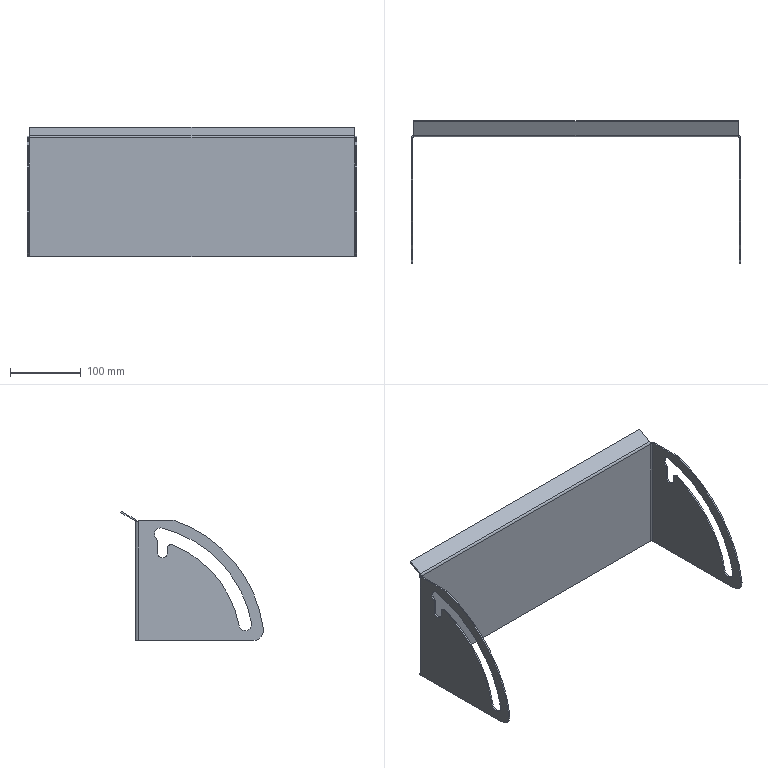Part | SolidWorks | features BaseBody 1 | 1 solid | 50 faces | box 465 x 201.23 x 182.5 mm | volume 260950 mm3 | cylinder 28 | plane 22 | commonest cylinder face diameters 18 x6 10 x4 30 x4 4 x3 8 x3 14 x2
STEP:
#1=CARTESIAN_POINT('',(-230.5,-162.198,-62.));
#2=VERTEX_POINT('',#1);
#3=CARTESIAN_POINT('',(-230.5,-162.042,-60.333));
#4=VERTEX_POINT('',#3);
#5=CARTESIAN_POINT('',(-230.5,-153.198,-62.));
#6=DIRECTION('',(-1.,0.,0.));
#7=DIRECTION('',(0.,-1.,0.));
#8=AXIS2_PLACEMENT_3D('',#5,#6,#7);
#9=CIRCLE('',#8,9.);
#10=EDGE_CURVE('',#2,#4,#9,.T.);
#11=ORIENTED_EDGE('',*,*,#10,.F.);
#12=CARTESIAN_POINT('',(-232.5,-162.198,-62.));
#13=VERTEX_POINT('',#12);
#14=CARTESIAN_POINT('',(232.5,-162.198,-62.));
#15=DIRECTION('',(-1.,0.,0.));
#16=VECTOR('',#15,1000.);
#17=LINE('',#14,#16);
#18=EDGE_CURVE('',#2,#13,#17,.T.);
#19=ORIENTED_EDGE('',*,*,#18,.T.);
#20=CARTESIAN_POINT('',(-232.5,-162.042,-60.333));
#21=VERTEX_POINT('',#20);
#22=CARTESIAN_POINT('',(-232.5,-153.198,-62.));
#23=DIRECTION('',(1.,0.,0.));
#24=DIRECTION('',(0.,-1.,0.));
#25=AXIS2_PLACEMENT_3D('',#22,#23,#24);
#26=CIRCLE('',#25,9.);
#27=EDGE_CURVE('',#21,#13,#26,.T.);
#28=ORIENTED_EDGE('',*,*,#27,.F.);
#29=CARTESIAN_POINT('',(232.5,-162.042,-60.333));
#30=DIRECTION('',(-1.,0.,0.));
#31=VECTOR('',#30,1000.);
#32=LINE('',#29,#31);
#33=EDGE_CURVE('',#4,#21,#32,.T.);
#34=ORIENTED_EDGE('',*,*,#33,.F.);
#35=EDGE_LOOP('',(#11,#19,#28,#34));
#36=FACE_OUTER_BOUND('',#35,.T.);
#37=CARTESIAN_POINT('',(232.5,-153.198,-62.));
#38=DIRECTION('',(-1.,0.,0.));
#39=DIRECTION('',(0.,-1.,0.));
#40=AXIS2_PLACEMENT_3D('',#37,#38,#39);
#41=CYLINDRICAL_SURFACE('',#40,9.);
#42=ADVANCED_FACE('',(#36),#41,.F.);
#43=CARTESIAN_POINT('',(-230.5,-163.579,-85.));
#44=VERTEX_POINT('',#43);
#45=CARTESIAN_POINT('',(-230.5,-178.579,-70.));
#46=VERTEX_POINT('',#45);
#47=CARTESIAN_POINT('',(-230.5,-163.579,-70.));
#48=DIRECTION('',(-1.,0.,0.));
#49=DIRECTION('',(0.,-1.,0.));
#50=AXIS2_PLACEMENT_3D('',#47,#48,#49);
#51=CIRCLE('',#50,15.);
#52=EDGE_CURVE('',#44,#46,#51,.T.);
#53=ORIENTED_EDGE('',*,*,#52,.T.);
#54=CARTESIAN_POINT('',(-232.5,-178.579,-70.));
#55=VERTEX_POINT('',#54);
#56=CARTESIAN_POINT('',(232.5,-178.579,-70.));
#57=DIRECTION('',(-1.,0.,0.));
#58=VECTOR('',#57,1000.);
#59=LINE('',#56,#58);
#60=EDGE_CURVE('',#46,#55,#59,.T.);
#61=ORIENTED_EDGE('',*,*,#60,.T.);
#62=CARTESIAN_POINT('',(-232.5,-163.579,-85.));
#63=VERTEX_POINT('',#62);
#64=CARTESIAN_POINT('',(-232.5,-163.579,-70.));
#65=DIRECTION('',(-1.,0.,0.));
#66=DIRECTION('',(0.,-1.,0.));
#67=AXIS2_PLACEMENT_3D('',#64,#65,#66);
#68=CIRCLE('',#67,15.);
#69=EDGE_CURVE('',#63,#55,#68,.T.);
#70=ORIENTED_EDGE('',*,*,#69,.F.);
#71=CARTESIAN_POINT('',(-230.5,-163.579,-85.));
#72=DIRECTION('',(-1.,0.,0.));
#73=VECTOR('',#72,1000.);
#74=LINE('',#71,#73);
#75=EDGE_CURVE('',#44,#63,#74,.T.);
#76=ORIENTED_EDGE('',*,*,#75,.F.);
#77=EDGE_LOOP('',(#53,#61,#70,#76));
#78=FACE_OUTER_BOUND('',#77,.T.);
#79=CARTESIAN_POINT('',(232.5,-163.579,-70.));
#80=DIRECTION('',(-1.,0.,0.));
#81=DIRECTION('',(0.,-1.,0.));
#82=AXIS2_PLACEMENT_3D('',#79,#80,#81);
#83=CYLINDRICAL_SURFACE('',#82,15.);
#84=ADVANCED_FACE('',(#78),#83,.T.);
#85=CARTESIAN_POINT('',(232.5,-162.198,-62.));
#86=VERTEX_POINT('',#85);
#87=CARTESIAN_POINT('',(232.5,-162.042,-60.333));
#88=VERTEX_POINT('',#87);
#89=CARTESIAN_POINT('',(232.5,-153.198,-62.));
#90=DIRECTION('',(-1.,0.,0.));
#91=DIRECTION('',(0.,-1.,0.));
#92=AXIS2_PLACEMENT_3D('',#89,#90,#91);
#93=CIRCLE('',#92,9.);
#94=EDGE_CURVE('',#86,#88,#93,.T.);
#95=ORIENTED_EDGE('',*,*,#94,.F.);
#96=CARTESIAN_POINT('',(230.5,-162.198,-62.));
#97=VERTEX_POINT('',#96);
#98=CARTESIAN_POINT('',(232.5,-162.198,-62.));
#99=DIRECTION('',(-1.,0.,0.));
#100=VECTOR('',#99,1000.);
#101=LINE('',#98,#100);
#102=EDGE_CURVE('',#86,#97,#101,.T.);
#103=ORIENTED_EDGE('',*,*,#102,.T.);
#104=CARTESIAN_POINT('',(230.5,-162.042,-60.333));
#105=VERTEX_POINT('',#104);
#106=CARTESIAN_POINT('',(230.5,-153.198,-62.));
#107=DIRECTION('',(1.,0.,0.));
#108=DIRECTION('',(0.,-1.,0.));
#109=AXIS2_PLACEMENT_3D('',#106,#107,#108);
#110=CIRCLE('',#109,9.);
#111=EDGE_CURVE('',#105,#97,#110,.T.);
#112=ORIENTED_EDGE('',*,*,#111,.F.);
#113=CARTESIAN_POINT('',(232.5,-162.042,-60.333));
#114=DIRECTION('',(1.,0.,0.));
#115=VECTOR('',#114,1000.);
#116=LINE('',#113,#115);
#117=EDGE_CURVE('',#105,#88,#116,.T.);
#118=ORIENTED_EDGE('',*,*,#117,.T.);
#119=EDGE_LOOP('',(#95,#103,#112,#118));
#120=FACE_OUTER_BOUND('',#119,.T.);
#121=CARTESIAN_POINT('',(232.5,-153.198,-62.));
#122=DIRECTION('',(-1.,0.,0.));
#123=DIRECTION('',(0.,-1.,0.));
#124=AXIS2_PLACEMENT_3D('',#121,#122,#123);
#125=CYLINDRICAL_SURFACE('',#124,9.);
#126=ADVANCED_FACE('',(#120),#125,.F.);
#127=CARTESIAN_POINT('',(232.5,-178.579,-70.));
#128=VERTEX_POINT('',#127);
#129=CARTESIAN_POINT('',(232.5,-163.579,-85.));
#130=VERTEX_POINT('',#129);
#131=CARTESIAN_POINT('',(232.5,-163.579,-70.));
#132=DIRECTION('',(1.,0.,0.));
#133=DIRECTION('',(0.,-1.,0.));
#134=AXIS2_PLACEMENT_3D('',#131,#132,#133);
#135=CIRCLE('',#134,15.);
#136=EDGE_CURVE('',#128,#130,#135,.T.);
#137=ORIENTED_EDGE('',*,*,#136,.F.);
#138=CARTESIAN_POINT('',(230.5,-178.579,-70.));
#139=VERTEX_POINT('',#138);
#140=CARTESIAN_POINT('',(232.5,-178.579,-70.));
#141=DIRECTION('',(-1.,0.,0.));
#142=VECTOR('',#141,1000.);
#143=LINE('',#140,#142);
#144=EDGE_CURVE('',#128,#139,#143,.T.);
#145=ORIENTED_EDGE('',*,*,#144,.T.);
#146=CARTESIAN_POINT('',(230.5,-163.579,-85.));
#147=VERTEX_POINT('',#146);
#148=CARTESIAN_POINT('',(230.5,-163.579,-70.));
#149=DIRECTION('',(1.,0.,0.));
#150=DIRECTION('',(0.,-1.,0.));
#151=AXIS2_PLACEMENT_3D('',#148,#149,#150);
#152=CIRCLE('',#151,15.);
#153=EDGE_CURVE('',#139,#147,#152,.T.);
#154=ORIENTED_EDGE('',*,*,#153,.T.);
#155=CARTESIAN_POINT('',(230.5,-163.579,-85.));
#156=DIRECTION('',(-1.,0.,0.));
#157=VECTOR('',#156,1000.);
#158=LINE('',#155,#157);
#159=EDGE_CURVE('',#130,#147,#158,.T.);
#160=ORIENTED_EDGE('',*,*,#159,.F.);
#161=EDGE_LOOP('',(#137,#145,#154,#160));
#162=FACE_OUTER_BOUND('',#161,.T.);
#163=CARTESIAN_POINT('',(232.5,-163.579,-70.));
#164=DIRECTION('',(-1.,0.,0.));
#165=DIRECTION('',(0.,-1.,0.));
#166=AXIS2_PLACEMENT_3D('',#163,#164,#165);
#167=CYLINDRICAL_SURFACE('',#166,15.);
#168=ADVANCED_FACE('',(#162),#167,.T.);
#169=CARTESIAN_POINT('',(228.5,2.,-85.));
#170=VERTEX_POINT('',#169);
#171=CARTESIAN_POINT('',(-228.5,2.,-85.));
#172=VERTEX_POINT('',#171);
#173=CARTESIAN_POINT('',(0.,2.,-85.));
#174=DIRECTION('',(-1.,0.,0.));
#175=VECTOR('',#174,1000.);
#176=LINE('',#173,#175);
#177=EDGE_CURVE('',#170,#172,#176,.T.);
#178=ORIENTED_EDGE('',*,*,#177,.T.);
#179=CARTESIAN_POINT('',(-228.5,2.,82.691));
#180=VERTEX_POINT('',#179);
#181=CARTESIAN_POINT('',(-228.5,2.,0.));
#182=DIRECTION('',(0.,0.,1.));
#183=VECTOR('',#182,1000.);
#184=LINE('',#181,#183);
#185=EDGE_CURVE('',#172,#180,#184,.T.);
#186=ORIENTED_EDGE('',*,*,#185,.T.);
#187=CARTESIAN_POINT('',(228.5,2.,82.691));
#188=VERTEX_POINT('',#187);
#189=CARTESIAN_POINT('',(0.,2.,82.691));
#190=DIRECTION('',(1.,0.,0.));
#191=VECTOR('',#190,1000.);
#192=LINE('',#189,#191);
#193=EDGE_CURVE('',#180,#188,#192,.T.);
#194=ORIENTED_EDGE('',*,*,#193,.T.);
#195=CARTESIAN_POINT('',(228.5,2.,0.));
#196=DIRECTION('',(0.,0.,-1.));
#197=VECTOR('',#196,1000.);
#198=LINE('',#195,#197);
#199=EDGE_CURVE('',#188,#170,#198,.T.);
#200=ORIENTED_EDGE('',*,*,#199,.T.);
#201=EDGE_LOOP('',(#178,#186,#194,#200));
#202=FACE_OUTER_BOUND('',#201,.T.);
#203=CARTESIAN_POINT('',(0.,2.,0.));
#204=DIRECTION('',(0.,1.,0.));
#205=DIRECTION('',(0.,0.,1.));
#206=AXIS2_PLACEMENT_3D('',#203,#204,#205);
#207=PLANE('',#206);
#208=ADVANCED_FACE('',(#202),#207,.T.);
#209=CARTESIAN_POINT('',(-232.5,-2.,-85.));
#210=VERTEX_POINT('',#209);
#211=CARTESIAN_POINT('',(-228.5,-2.,-85.));
#212=DIRECTION('',(0.,0.,1.));
#213=DIRECTION('',(1.,0.,0.));
#214=AXIS2_PLACEMENT_3D('',#211,#212,#213);
#215=CIRCLE('',#214,4.);
#216=EDGE_CURVE('',#172,#210,#215,.T.);
#217=ORIENTED_EDGE('',*,*,#216,.T.);
#218=CARTESIAN_POINT('',(-232.5,-2.,82.691));
#219=VERTEX_POINT('',#218);
#220=CARTESIAN_POINT('',(-232.5,-2.,0.));
#221=DIRECTION('',(0.,0.,1.));
#222=VECTOR('',#221,1000.);
#223=LINE('',#220,#222);
#224=EDGE_CURVE('',#210,#219,#223,.T.);
#225=ORIENTED_EDGE('',*,*,#224,.T.);
#226=CARTESIAN_POINT('',(-228.5,-2.,82.691));
#227=DIRECTION('',(0.,0.,-1.));
#228=DIRECTION('',(1.,0.,0.));
#229=AXIS2_PLACEMENT_3D('',#226,#227,#228);
#230=CIRCLE('',#229,4.);
#231=EDGE_CURVE('',#219,#180,#230,.T.);
#232=ORIENTED_EDGE('',*,*,#231,.T.);
#233=ORIENTED_EDGE('',*,*,#185,.F.);
#234=EDGE_LOOP('',(#217,#225,#232,#233));
#235=FACE_OUTER_BOUND('',#234,.T.);
#236=CARTESIAN_POINT('',(-228.5,-2.,0.));
#237=DIRECTION('',(0.,0.,1.));
#238=DIRECTION('',(1.,0.,0.));
#239=AXIS2_PLACEMENT_3D('',#236,#237,#238);
#240=CYLINDRICAL_SURFACE('',#239,4.);
#241=ADVANCED_FACE('',(#235),#240,.T.);
#242=ORIENTED_EDGE('',*,*,#177,.F.);
#243=CARTESIAN_POINT('',(232.5,-2.,-85.));
#244=VERTEX_POINT('',#243);
#245=CARTESIAN_POINT('',(228.5,-2.,-85.));
#246=DIRECTION('',(0.,0.,1.));
#247=DIRECTION('',(-1.,0.,0.));
#248=AXIS2_PLACEMENT_3D('',#245,#246,#247);
#249=CIRCLE('',#248,4.);
#250=EDGE_CURVE('',#244,#170,#249,.T.);
#251=ORIENTED_EDGE('',*,*,#250,.F.);
#252=CARTESIAN_POINT('',(232.5,-88.738,-85.));
#253=DIRECTION('',(0.,1.,0.));
#254=VECTOR('',#253,1000.);
#255=LINE('',#252,#254);
#256=EDGE_CURVE('',#130,#244,#255,.T.);
#257=ORIENTED_EDGE('',*,*,#256,.F.);
#258=ORIENTED_EDGE('',*,*,#159,.T.);
#259=CARTESIAN_POINT('',(230.5,-2.,-85.));
#260=VERTEX_POINT('',#259);
#261=CARTESIAN_POINT('',(230.5,-2.,-85.));
#262=DIRECTION('',(0.,1.,0.));
#263=VECTOR('',#262,1000.);
#264=LINE('',#261,#263);
#265=EDGE_CURVE('',#147,#260,#264,.T.);
#266=ORIENTED_EDGE('',*,*,#265,.T.);
#267=CARTESIAN_POINT('',(228.5,0.,-85.));
#268=VERTEX_POINT('',#267);
#269=CARTESIAN_POINT('',(228.5,-2.,-85.));
#270=DIRECTION('',(0.,0.,1.));
#271=DIRECTION('',(-1.,0.,0.));
#272=AXIS2_PLACEMENT_3D('',#269,#270,#271);
#273=CIRCLE('',#272,2.);
#274=EDGE_CURVE('',#260,#268,#273,.T.);
#275=ORIENTED_EDGE('',*,*,#274,.T.);
#276=CARTESIAN_POINT('',(-228.5,0.,-85.));
#277=VERTEX_POINT('',#276);
#278=CARTESIAN_POINT('',(-232.5,0.,-85.));
#279=DIRECTION('',(-1.,0.,0.));
#280=VECTOR('',#279,1000.);
#281=LINE('',#278,#280);
#282=EDGE_CURVE('',#268,#277,#281,.T.);
#283=ORIENTED_EDGE('',*,*,#282,.T.);
#284=CARTESIAN_POINT('',(-230.5,-2.,-85.));
#285=VERTEX_POINT('',#284);
#286=CARTESIAN_POINT('',(-228.5,-2.,-85.));
#287=DIRECTION('',(0.,0.,1.));
#288=DIRECTION('',(1.,0.,0.));
#289=AXIS2_PLACEMENT_3D('',#286,#287,#288);
#290=CIRCLE('',#289,2.);
#291=EDGE_CURVE('',#277,#285,#290,.T.);
#292=ORIENTED_EDGE('',*,*,#291,.T.);
#293=CARTESIAN_POINT('',(-230.5,-2.,-85.));
#294=DIRECTION('',(0.,-1.,0.));
#295=VECTOR('',#294,1000.);
#296=LINE('',#293,#295);
#297=EDGE_CURVE('',#285,#44,#296,.T.);
#298=ORIENTED_EDGE('',*,*,#297,.T.);
#299=ORIENTED_EDGE('',*,*,#75,.T.);
#300=CARTESIAN_POINT('',(-232.5,-88.738,-85.));
#301=DIRECTION('',(0.,-1.,0.));
#302=VECTOR('',#301,1000.);
#303=LINE('',#300,#302);
#304=EDGE_CURVE('',#210,#63,#303,.T.);
#305=ORIENTED_EDGE('',*,*,#304,.F.);
#306=ORIENTED_EDGE('',*,*,#216,.F.);
#307=EDGE_LOOP('',(#242,#251,#257,#258,#266,#275,#283,#292,#298,#299,#305,#306));
#308=FACE_OUTER_BOUND('',#307,.T.);
#309=CARTESIAN_POINT('',(-232.5,0.,-85.));
#310=DIRECTION('',(0.,0.,-1.));
#311=DIRECTION('',(-1.,0.,0.));
#312=AXIS2_PLACEMENT_3D('',#309,#310,#311);
#313=PLANE('',#312);
#314=ADVANCED_FACE('',(#308),#313,.T.);
#315=ORIENTED_EDGE('',*,*,#250,.T.);
#316=ORIENTED_EDGE('',*,*,#199,.F.);
#317=CARTESIAN_POINT('',(232.5,-2.,82.691));
#318=VERTEX_POINT('',#317);
#319=CARTESIAN_POINT('',(228.5,-2.,82.691));
#320=DIRECTION('',(0.,0.,-1.));
#321=DIRECTION('',(-1.,0.,0.));
#322=AXIS2_PLACEMENT_3D('',#319,#320,#321);
#323=CIRCLE('',#322,4.);
#324=EDGE_CURVE('',#188,#318,#323,.T.);
#325=ORIENTED_EDGE('',*,*,#324,.T.);
#326=CARTESIAN_POINT('',(232.5,-2.,0.));
#327=DIRECTION('',(0.,0.,-1.));
#328=VECTOR('',#327,1000.);
#329=LINE('',#326,#328);
#330=EDGE_CURVE('',#318,#244,#329,.T.);
#331=ORIENTED_EDGE('',*,*,#330,.T.);
#332=EDGE_LOOP('',(#315,#316,#325,#331));
#333=FACE_OUTER_BOUND('',#332,.T.);
#334=CARTESIAN_POINT('',(228.5,-2.,0.));
#335=DIRECTION('',(0.,0.,-1.));
#336=DIRECTION('',(-1.,0.,0.));
#337=AXIS2_PLACEMENT_3D('',#334,#335,#336);
#338=CYLINDRICAL_SURFACE('',#337,4.);
#339=ADVANCED_FACE('',(#333),#338,.T.);
#340=CARTESIAN_POINT('',(228.5,3.,84.423));
#341=VERTEX_POINT('',#340);
#342=CARTESIAN_POINT('',(228.5,4.,82.691));
#343=DIRECTION('',(-1.,0.,0.));
#344=DIRECTION('',(0.,0.,1.));
#345=AXIS2_PLACEMENT_3D('',#342,#343,#344);
#346=CIRCLE('',#345,2.);
#347=EDGE_CURVE('',#188,#341,#346,.T.);
#348=ORIENTED_EDGE('',*,*,#347,.F.);
#349=ORIENTED_EDGE('',*,*,#193,.F.);
#350=CARTESIAN_POINT('',(-228.5,3.,84.423));
#351=VERTEX_POINT('',#350);
#352=CARTESIAN_POINT('',(-228.5,4.,82.691));
#353=DIRECTION('',(1.,0.,0.));
#354=DIRECTION('',(0.,0.,1.));
#355=AXIS2_PLACEMENT_3D('',#352,#353,#354);
#356=CIRCLE('',#355,2.);
#357=EDGE_CURVE('',#351,#180,#356,.T.);
#358=ORIENTED_EDGE('',*,*,#357,.F.);
#359=CARTESIAN_POINT('',(0.,3.,84.423));
#360=DIRECTION('',(-1.,0.,0.));
#361=VECTOR('',#360,1000.);
#362=LINE('',#359,#361);
#363=EDGE_CURVE('',#341,#351,#362,.T.);
#364=ORIENTED_EDGE('',*,*,#363,.F.);
#365=EDGE_LOOP('',(#348,#349,#358,#364));
#366=FACE_OUTER_BOUND('',#365,.T.);
#367=CARTESIAN_POINT('',(0.,4.,82.691));
#368=DIRECTION('',(-1.,0.,0.));
#369=DIRECTION('',(0.,0.,1.));
#370=AXIS2_PLACEMENT_3D('',#367,#368,#369);
#371=CYLINDRICAL_SURFACE('',#370,2.);
#372=ADVANCED_FACE('',(#366),#371,.F.);
#373=ORIENTED_EDGE('',*,*,#27,.T.);
#374=CARTESIAN_POINT('',(-232.5,-144.354,-63.667));
#375=VERTEX_POINT('',#374);
#376=CARTESIAN_POINT('',(-232.5,-153.198,-62.));
#377=DIRECTION('',(1.,0.,0.));
#378=DIRECTION('',(0.,-1.,0.));
#379=AXIS2_PLACEMENT_3D('',#376,#377,#378);
#380=CIRCLE('',#379,9.);
#381=EDGE_CURVE('',#13,#375,#380,.T.);
#382=ORIENTED_EDGE('',*,*,#381,.T.);
#383=CARTESIAN_POINT('',(-232.5,-50.205,50.303));
#384=VERTEX_POINT('',#383);
#385=CARTESIAN_POINT('',(-232.5,6.,-92.));
#386=DIRECTION('',(-1.,0.,0.));
#387=DIRECTION('',(0.,-1.,0.));
#388=AXIS2_PLACEMENT_3D('',#385,#386,#387);
#389=CIRCLE('',#388,153.);
#390=EDGE_CURVE('',#375,#384,#389,.T.);
#391=ORIENTED_EDGE('',*,*,#390,.T.);
#392=CARTESIAN_POINT('',(-232.5,-43.368,45.652));
#393=VERTEX_POINT('',#392);
#394=CARTESIAN_POINT('',(-232.5,-48.368,45.652));
#395=DIRECTION('',(-1.,0.,0.));
#396=DIRECTION('',(0.,-1.,0.));
#397=AXIS2_PLACEMENT_3D('',#394,#395,#396);
#398=CIRCLE('',#397,5.);
#399=EDGE_CURVE('',#384,#393,#398,.T.);
#400=ORIENTED_EDGE('',*,*,#399,.T.);
#401=CARTESIAN_POINT('',(-232.5,-43.368,39.017));
#402=VERTEX_POINT('',#401);
#403=CARTESIAN_POINT('',(-232.5,-43.368,0.));
#404=DIRECTION('',(0.,0.,-1.));
#405=VECTOR('',#404,1000.);
#406=LINE('',#403,#405);
#407=EDGE_CURVE('',#393,#402,#406,.T.);
#408=ORIENTED_EDGE('',*,*,#407,.T.);
#409=CARTESIAN_POINT('',(-232.5,-29.368,39.017));
#410=VERTEX_POINT('',#409);
#411=CARTESIAN_POINT('',(-232.5,-36.368,39.017));
#412=DIRECTION('',(1.,0.,0.));
#413=DIRECTION('',(0.,-1.,0.));
#414=AXIS2_PLACEMENT_3D('',#411,#412,#413);
#415=CIRCLE('',#414,7.);
#416=EDGE_CURVE('',#402,#410,#415,.T.);
#417=ORIENTED_EDGE('',*,*,#416,.T.);
#418=CARTESIAN_POINT('',(-232.5,-29.368,54.824));
#419=VERTEX_POINT('',#418);
#420=CARTESIAN_POINT('',(-232.5,-29.368,0.));
#421=DIRECTION('',(0.,0.,1.));
#422=VECTOR('',#421,1000.);
#423=LINE('',#420,#422);
#424=EDGE_CURVE('',#410,#419,#423,.T.);
#425=ORIENTED_EDGE('',*,*,#424,.T.);
#426=CARTESIAN_POINT('',(-232.5,-27.808,58.453));
#427=VERTEX_POINT('',#426);
#428=CARTESIAN_POINT('',(-232.5,-24.368,54.824));
#429=DIRECTION('',(-1.,0.,0.));
#430=DIRECTION('',(0.,-1.,0.));
#431=AXIS2_PLACEMENT_3D('',#428,#429,#430);
#432=CIRCLE('',#431,5.);
#433=EDGE_CURVE('',#419,#427,#432,.T.);
#434=ORIENTED_EDGE('',*,*,#433,.T.);
#435=CARTESIAN_POINT('',(-232.5,-36.222,73.705));
#436=VERTEX_POINT('',#435);
#437=CARTESIAN_POINT('',(-232.5,-34.,64.984));
#438=DIRECTION('',(1.,0.,0.));
#439=DIRECTION('',(0.,-1.,0.));
#440=AXIS2_PLACEMENT_3D('',#437,#438,#439);
#441=CIRCLE('',#440,9.);
#442=EDGE_CURVE('',#427,#436,#441,.T.);
#443=ORIENTED_EDGE('',*,*,#442,.T.);
#444=CARTESIAN_POINT('',(-232.5,6.,-92.));
#445=DIRECTION('',(1.,0.,0.));
#446=DIRECTION('',(0.,-1.,0.));
#447=AXIS2_PLACEMENT_3D('',#444,#445,#446);
#448=CIRCLE('',#447,171.);
#449=EDGE_CURVE('',#436,#21,#448,.T.);
#450=ORIENTED_EDGE('',*,*,#449,.T.);
#451=EDGE_LOOP('',(#373,#382,#391,#400,#408,#417,#425,#434,#443,#450));
#452=FACE_BOUND('',#451,.T.);
#453=ORIENTED_EDGE('',*,*,#224,.F.);
#454=ORIENTED_EDGE('',*,*,#304,.T.);
#455=ORIENTED_EDGE('',*,*,#69,.T.);
#456=CARTESIAN_POINT('',(-232.5,-178.454,-68.07));
#457=VERTEX_POINT('',#456);
#458=CARTESIAN_POINT('',(-232.5,-163.579,-70.));
#459=DIRECTION('',(-1.,0.,0.));
#460=DIRECTION('',(0.,-1.,0.));
#461=AXIS2_PLACEMENT_3D('',#458,#459,#460);
#462=CIRCLE('',#461,15.);
#463=EDGE_CURVE('',#55,#457,#462,.T.);
#464=ORIENTED_EDGE('',*,*,#463,.T.);
#465=CARTESIAN_POINT('',(-232.5,-51.158,85.));
#466=VERTEX_POINT('',#465);
#467=CARTESIAN_POINT('',(-232.5,6.,-92.));
#468=DIRECTION('',(-1.,0.,0.));
#469=DIRECTION('',(0.,-1.,0.));
#470=AXIS2_PLACEMENT_3D('',#467,#468,#469);
#471=CIRCLE('',#470,186.);
#472=EDGE_CURVE('',#457,#466,#471,.T.);
#473=ORIENTED_EDGE('',*,*,#472,.T.);
#474=CARTESIAN_POINT('',(-232.5,-2.,85.));
#475=VERTEX_POINT('',#474);
#476=CARTESIAN_POINT('',(-232.5,-88.738,85.));
#477=DIRECTION('',(0.,1.,0.));
#478=VECTOR('',#477,1000.);
#479=LINE('',#476,#478);
#480=EDGE_CURVE('',#466,#475,#479,.T.);
#481=ORIENTED_EDGE('',*,*,#480,.T.);
#482=CARTESIAN_POINT('',(-232.5,-2.,0.));
#483=DIRECTION('',(0.,0.,-1.));
#484=VECTOR('',#483,1000.);
#485=LINE('',#482,#484);
#486=EDGE_CURVE('',#475,#219,#485,.T.);
#487=ORIENTED_EDGE('',*,*,#486,.T.);
#488=EDGE_LOOP('',(#453,#454,#455,#464,#473,#481,#487));
#489=FACE_OUTER_BOUND('',#488,.T.);
#490=CARTESIAN_POINT('',(-232.5,-88.738,0.));
#491=DIRECTION('',(-1.,0.,0.));
#492=DIRECTION('',(0.,-1.,0.));
#493=AXIS2_PLACEMENT_3D('',#490,#491,#492);
#494=PLANE('',#493);
#495=ADVANCED_FACE('',(#452,#489),#494,.T.);
#496=CARTESIAN_POINT('',(-230.5,-2.,82.691));
#497=VERTEX_POINT('',#496);
#498=CARTESIAN_POINT('',(-228.5,0.,82.691));
#499=VERTEX_POINT('',#498);
#500=CARTESIAN_POINT('',(-228.5,-2.,82.691));
#501=DIRECTION('',(0.,0.,-1.));
#502=DIRECTION('',(1.,0.,0.));
#503=AXIS2_PLACEMENT_3D('',#500,#501,#502);
#504=CIRCLE('',#503,2.);
#505=EDGE_CURVE('',#497,#499,#504,.T.);
#506=ORIENTED_EDGE('',*,*,#505,.T.);
#507=CARTESIAN_POINT('',(-228.5,-0.09513,82.691));
#508=DIRECTION('',(0.,1.,0.));
#509=VECTOR('',#508,1000.);
#510=LINE('',#507,#509);
#511=EDGE_CURVE('',#499,#180,#510,.T.);
#512=ORIENTED_EDGE('',*,*,#511,.T.);
#513=ORIENTED_EDGE('',*,*,#231,.F.);
#514=CARTESIAN_POINT('',(-230.405,-2.,82.691));
#515=DIRECTION('',(1.,0.,0.));
#516=VECTOR('',#515,1000.);
#517=LINE('',#514,#516);
#518=EDGE_CURVE('',#219,#497,#517,.T.);
#519=ORIENTED_EDGE('',*,*,#518,.T.);
#520=EDGE_LOOP('',(#506,#512,#513,#519));
#521=FACE_OUTER_BOUND('',#520,.T.);
#522=CARTESIAN_POINT('',(-230.405,-0.09513,82.691));
#523=DIRECTION('',(0.,0.,1.));
#524=DIRECTION('',(1.,0.,0.));
#525=AXIS2_PLACEMENT_3D('',#522,#523,#524);
#526=PLANE('',#525);
#527=ADVANCED_FACE('',(#521),#526,.T.);
#528=CARTESIAN_POINT('',(-228.5,0.,0.));
#529=DIRECTION('',(0.,0.,1.));
#530=VECTOR('',#529,1000.);
#531=LINE('',#528,#530);
#532=EDGE_CURVE('',#277,#499,#531,.T.);
#533=ORIENTED_EDGE('',*,*,#532,.F.);
#534=ORIENTED_EDGE('',*,*,#282,.F.);
#535=CARTESIAN_POINT('',(228.5,0.,82.691));
#536=VERTEX_POINT('',#535);
#537=CARTESIAN_POINT('',(228.5,0.,0.));
#538=DIRECTION('',(0.,0.,-1.));
#539=VECTOR('',#538,1000.);
#540=LINE('',#537,#539);
#541=EDGE_CURVE('',#536,#268,#540,.T.);
#542=ORIENTED_EDGE('',*,*,#541,.F.);
#543=CARTESIAN_POINT('',(0.,0.,82.691));
#544=DIRECTION('',(1.,0.,0.));
#545=VECTOR('',#544,1000.);
#546=LINE('',#543,#545);
#547=EDGE_CURVE('',#499,#536,#546,.T.);
#548=ORIENTED_EDGE('',*,*,#547,.F.);
#549=EDGE_LOOP('',(#533,#534,#542,#548));
#550=FACE_OUTER_BOUND('',#549,.T.);
#551=CARTESIAN_POINT('',(0.,0.,0.));
#552=DIRECTION('',(0.,1.,0.));
#553=DIRECTION('',(0.,0.,1.));
#554=AXIS2_PLACEMENT_3D('',#551,#552,#553);
#555=PLANE('',#554);
#556=ADVANCED_FACE('',(#550),#555,.F.);
#557=CARTESIAN_POINT('',(232.5,-36.222,73.705));
#558=VERTEX_POINT('',#557);
#559=CARTESIAN_POINT('',(232.5,6.,-92.));
#560=DIRECTION('',(-1.,0.,0.));
#561=DIRECTION('',(0.,-1.,0.));
#562=AXIS2_PLACEMENT_3D('',#559,#560,#561);
#563=CIRCLE('',#562,171.);
#564=EDGE_CURVE('',#88,#558,#563,.T.);
#565=ORIENTED_EDGE('',*,*,#564,.T.);
#566=CARTESIAN_POINT('',(232.5,-27.808,58.453));
#567=VERTEX_POINT('',#566);
#568=CARTESIAN_POINT('',(232.5,-34.,64.984));
#569=DIRECTION('',(-1.,0.,0.));
#570=DIRECTION('',(0.,-1.,0.));
#571=AXIS2_PLACEMENT_3D('',#568,#569,#570);
#572=CIRCLE('',#571,9.);
#573=EDGE_CURVE('',#558,#567,#572,.T.);
#574=ORIENTED_EDGE('',*,*,#573,.T.);
#575=CARTESIAN_POINT('',(232.5,-29.368,54.824));
#576=VERTEX_POINT('',#575);
#577=CARTESIAN_POINT('',(232.5,-24.368,54.824));
#578=DIRECTION('',(1.,0.,0.));
#579=DIRECTION('',(0.,-1.,0.));
#580=AXIS2_PLACEMENT_3D('',#577,#578,#579);
#581=CIRCLE('',#580,5.);
#582=EDGE_CURVE('',#567,#576,#581,.T.);
#583=ORIENTED_EDGE('',*,*,#582,.T.);
#584=CARTESIAN_POINT('',(232.5,-29.368,39.017));
#585=VERTEX_POINT('',#584);
#586=CARTESIAN_POINT('',(232.5,-29.368,0.));
#587=DIRECTION('',(0.,0.,-1.));
#588=VECTOR('',#587,1000.);
#589=LINE('',#586,#588);
#590=EDGE_CURVE('',#576,#585,#589,.T.);
#591=ORIENTED_EDGE('',*,*,#590,.T.);
#592=CARTESIAN_POINT('',(232.5,-43.368,39.017));
#593=VERTEX_POINT('',#592);
#594=CARTESIAN_POINT('',(232.5,-36.368,39.017));
#595=DIRECTION('',(-1.,0.,0.));
#596=DIRECTION('',(0.,-1.,0.));
#597=AXIS2_PLACEMENT_3D('',#594,#595,#596);
#598=CIRCLE('',#597,7.);
#599=EDGE_CURVE('',#585,#593,#598,.T.);
#600=ORIENTED_EDGE('',*,*,#599,.T.);
#601=CARTESIAN_POINT('',(232.5,-43.368,45.652));
#602=VERTEX_POINT('',#601);
#603=CARTESIAN_POINT('',(232.5,-43.368,0.));
#604=DIRECTION('',(0.,0.,1.));
#605=VECTOR('',#604,1000.);
#606=LINE('',#603,#605);
#607=EDGE_CURVE('',#593,#602,#606,.T.);
#608=ORIENTED_EDGE('',*,*,#607,.T.);
#609=CARTESIAN_POINT('',(232.5,-50.205,50.303));
#610=VERTEX_POINT('',#609);
#611=CARTESIAN_POINT('',(232.5,-48.368,45.652));
#612=DIRECTION('',(1.,0.,0.));
#613=DIRECTION('',(0.,-1.,0.));
#614=AXIS2_PLACEMENT_3D('',#611,#612,#613);
#615=CIRCLE('',#614,5.);
#616=EDGE_CURVE('',#602,#610,#615,.T.);
#617=ORIENTED_EDGE('',*,*,#616,.T.);
#618=CARTESIAN_POINT('',(232.5,-144.354,-63.667));
#619=VERTEX_POINT('',#618);
#620=CARTESIAN_POINT('',(232.5,6.,-92.));
#621=DIRECTION('',(1.,0.,0.));
#622=DIRECTION('',(0.,-1.,0.));
#623=AXIS2_PLACEMENT_3D('',#620,#621,#622);
#624=CIRCLE('',#623,153.);
#625=EDGE_CURVE('',#610,#619,#624,.T.);
#626=ORIENTED_EDGE('',*,*,#625,.T.);
#627=CARTESIAN_POINT('',(232.5,-153.198,-62.));
#628=DIRECTION('',(-1.,0.,0.));
#629=DIRECTION('',(0.,-1.,0.));
#630=AXIS2_PLACEMENT_3D('',#627,#628,#629);
#631=CIRCLE('',#630,9.);
#632=EDGE_CURVE('',#619,#86,#631,.T.);
#633=ORIENTED_EDGE('',*,*,#632,.T.);
#634=ORIENTED_EDGE('',*,*,#94,.T.);
#635=EDGE_LOOP('',(#565,#574,#583,#591,#600,#608,#617,#626,#633,#634));
#636=FACE_BOUND('',#635,.T.);
#637=CARTESIAN_POINT('',(232.5,-2.,85.));
#638=VERTEX_POINT('',#637);
#639=CARTESIAN_POINT('',(232.5,-51.158,85.));
#640=VERTEX_POINT('',#639);
#641=CARTESIAN_POINT('',(232.5,-88.738,85.));
#642=DIRECTION('',(0.,-1.,0.));
#643=VECTOR('',#642,1000.);
#644=LINE('',#641,#643);
#645=EDGE_CURVE('',#638,#640,#644,.T.);
#646=ORIENTED_EDGE('',*,*,#645,.T.);
#647=CARTESIAN_POINT('',(232.5,-178.454,-68.07));
#648=VERTEX_POINT('',#647);
#649=CARTESIAN_POINT('',(232.5,6.,-92.));
#650=DIRECTION('',(1.,0.,0.));
#651=DIRECTION('',(0.,-1.,0.));
#652=AXIS2_PLACEMENT_3D('',#649,#650,#651);
#653=CIRCLE('',#652,186.);
#654=EDGE_CURVE('',#640,#648,#653,.T.);
#655=ORIENTED_EDGE('',*,*,#654,.T.);
#656=CARTESIAN_POINT('',(232.5,-163.579,-70.));
#657=DIRECTION('',(1.,0.,0.));
#658=DIRECTION('',(0.,-1.,0.));
#659=AXIS2_PLACEMENT_3D('',#656,#657,#658);
#660=CIRCLE('',#659,15.);
#661=EDGE_CURVE('',#648,#128,#660,.T.);
#662=ORIENTED_EDGE('',*,*,#661,.T.);
#663=ORIENTED_EDGE('',*,*,#136,.T.);
#664=ORIENTED_EDGE('',*,*,#256,.T.);
#665=ORIENTED_EDGE('',*,*,#330,.F.);
#666=CARTESIAN_POINT('',(232.5,-2.,0.));
#667=DIRECTION('',(0.,0.,1.));
#668=VECTOR('',#667,1000.);
#669=LINE('',#666,#668);
#670=EDGE_CURVE('',#318,#638,#669,.T.);
#671=ORIENTED_EDGE('',*,*,#670,.T.);
#672=EDGE_LOOP('',(#646,#655,#662,#663,#664,#665,#671));
#673=FACE_OUTER_BOUND('',#672,.T.);
#674=CARTESIAN_POINT('',(232.5,-88.738,0.));
#675=DIRECTION('',(1.,0.,0.));
#676=DIRECTION('',(0.,1.,0.));
#677=AXIS2_PLACEMENT_3D('',#674,#675,#676);
#678=PLANE('',#677);
#679=ADVANCED_FACE('',(#636,#673),#678,.T.);
#680=CARTESIAN_POINT('',(230.5,-2.,82.691));
#681=VERTEX_POINT('',#680);
#682=CARTESIAN_POINT('',(228.5,-2.,82.691));
#683=DIRECTION('',(0.,0.,-1.));
#684=DIRECTION('',(-1.,0.,0.));
#685=AXIS2_PLACEMENT_3D('',#682,#683,#684);
#686=CIRCLE('',#685,2.);
#687=EDGE_CURVE('',#536,#681,#686,.T.);
#688=ORIENTED_EDGE('',*,*,#687,.T.);
#689=CARTESIAN_POINT('',(230.405,-2.,82.691));
#690=DIRECTION('',(1.,0.,0.));
#691=VECTOR('',#690,1000.);
#692=LINE('',#689,#691);
#693=EDGE_CURVE('',#681,#318,#692,.T.);
#694=ORIENTED_EDGE('',*,*,#693,.T.);
#695=ORIENTED_EDGE('',*,*,#324,.F.);
#696=CARTESIAN_POINT('',(228.5,-0.09513,82.691));
#697=DIRECTION('',(0.,-1.,0.));
#698=VECTOR('',#697,1000.);
#699=LINE('',#696,#698);
#700=EDGE_CURVE('',#188,#536,#699,.T.);
#701=ORIENTED_EDGE('',*,*,#700,.T.);
#702=EDGE_LOOP('',(#688,#694,#695,#701));
#703=FACE_OUTER_BOUND('',#702,.T.);
#704=CARTESIAN_POINT('',(230.405,-0.09513,82.691));
#705=DIRECTION('',(0.,0.,1.));
#706=DIRECTION('',(1.,0.,0.));
#707=AXIS2_PLACEMENT_3D('',#704,#705,#706);
#708=PLANE('',#707);
#709=ADVANCED_FACE('',(#703),#708,.T.);
#710=CARTESIAN_POINT('',(-228.5,22.651,95.768));
#711=VERTEX_POINT('',#710);
#712=CARTESIAN_POINT('',(228.5,22.651,95.768));
#713=VERTEX_POINT('',#712);
#714=CARTESIAN_POINT('',(0.,22.651,95.768));
#715=DIRECTION('',(1.,0.,0.));
#716=VECTOR('',#715,1000.);
#717=LINE('',#714,#716);
#718=EDGE_CURVE('',#711,#713,#717,.T.);
#719=ORIENTED_EDGE('',*,*,#718,.T.);
#720=CARTESIAN_POINT('',(228.5,11.519,89.341));
#721=DIRECTION('',(0.,-0.866,-0.5));
#722=VECTOR('',#721,1000.);
#723=LINE('',#720,#722);
#724=EDGE_CURVE('',#713,#341,#723,.T.);
#725=ORIENTED_EDGE('',*,*,#724,.T.);
#726=ORIENTED_EDGE('',*,*,#363,.T.);
#727=CARTESIAN_POINT('',(-228.5,11.519,89.341));
#728=DIRECTION('',(0.,0.866,0.5));
#729=VECTOR('',#728,1000.);
#730=LINE('',#727,#729);
#731=EDGE_CURVE('',#351,#711,#730,.T.);
#732=ORIENTED_EDGE('',*,*,#731,.T.);
#733=EDGE_LOOP('',(#719,#725,#726,#732));
#734=FACE_OUTER_BOUND('',#733,.T.);
#735=CARTESIAN_POINT('',(0.,11.519,89.341));
#736=DIRECTION('',(0.,0.5,-0.866));
#737=DIRECTION('',(0.,0.866,0.5));
#738=AXIS2_PLACEMENT_3D('',#735,#736,#737);
#739=PLANE('',#738);
#740=ADVANCED_FACE('',(#734),#739,.T.);
#741=ORIENTED_EDGE('',*,*,#700,.F.);
#742=ORIENTED_EDGE('',*,*,#347,.T.);
#743=ORIENTED_EDGE('',*,*,#724,.F.);
#744=CARTESIAN_POINT('',(228.5,21.651,97.5));
#745=VERTEX_POINT('',#744);
#746=CARTESIAN_POINT('',(228.5,22.651,95.768));
#747=DIRECTION('',(0.,-0.5,0.866));
#748=VECTOR('',#747,1000.);
#749=LINE('',#746,#748);
#750=EDGE_CURVE('',#713,#745,#749,.T.);
#751=ORIENTED_EDGE('',*,*,#750,.T.);
#752=CARTESIAN_POINT('',(228.5,2.,86.155));
#753=VERTEX_POINT('',#752);
#754=CARTESIAN_POINT('',(228.5,21.651,97.5));
#755=DIRECTION('',(0.,-0.866,-0.5));
#756=VECTOR('',#755,1000.);
#757=LINE('',#754,#756);
#758=EDGE_CURVE('',#745,#753,#757,.T.);
#759=ORIENTED_EDGE('',*,*,#758,.T.);
#760=CARTESIAN_POINT('',(228.5,4.,82.691));
#761=DIRECTION('',(1.,0.,0.));
#762=DIRECTION('',(0.,0.,1.));
#763=AXIS2_PLACEMENT_3D('',#760,#761,#762);
#764=CIRCLE('',#763,4.);
#765=EDGE_CURVE('',#753,#536,#764,.T.);
#766=ORIENTED_EDGE('',*,*,#765,.T.);
#767=EDGE_LOOP('',(#741,#742,#743,#751,#759,#766));
#768=FACE_OUTER_BOUND('',#767,.T.);
#769=CARTESIAN_POINT('',(228.5,2.,86.155));
#770=DIRECTION('',(1.,0.,0.));
#771=DIRECTION('',(0.,0.,-1.));
#772=AXIS2_PLACEMENT_3D('',#769,#770,#771);
#773=PLANE('',#772);
#774=ADVANCED_FACE('',(#768),#773,.T.);
#775=ORIENTED_EDGE('',*,*,#511,.F.);
#776=CARTESIAN_POINT('',(-228.5,2.,86.155));
#777=VERTEX_POINT('',#776);
#778=CARTESIAN_POINT('',(-228.5,4.,82.691));
#779=DIRECTION('',(-1.,0.,0.));
#780=DIRECTION('',(0.,0.,1.));
#781=AXIS2_PLACEMENT_3D('',#778,#779,#780);
#782=CIRCLE('',#781,4.);
#783=EDGE_CURVE('',#499,#777,#782,.T.);
#784=ORIENTED_EDGE('',*,*,#783,.T.);
#785=CARTESIAN_POINT('',(-228.5,21.651,97.5));
#786=VERTEX_POINT('',#785);
#787=CARTESIAN_POINT('',(-228.5,2.,86.155));
#788=DIRECTION('',(0.,0.866,0.5));
#789=VECTOR('',#788,1000.);
#790=LINE('',#787,#789);
#791=EDGE_CURVE('',#777,#786,#790,.T.);
#792=ORIENTED_EDGE('',*,*,#791,.T.);
#793=CARTESIAN_POINT('',(-228.5,22.651,95.768));
#794=DIRECTION('',(0.,-0.5,0.866));
#795=VECTOR('',#794,1000.);
#796=LINE('',#793,#795);
#797=EDGE_CURVE('',#711,#786,#796,.T.);
#798=ORIENTED_EDGE('',*,*,#797,.F.);
#799=ORIENTED_EDGE('',*,*,#731,.F.);
#800=ORIENTED_EDGE('',*,*,#357,.T.);
#801=EDGE_LOOP('',(#775,#784,#792,#798,#799,#800));
#802=FACE_OUTER_BOUND('',#801,.T.);
#803=CARTESIAN_POINT('',(-228.5,3.,84.423));
#804=DIRECTION('',(-1.,0.,0.));
#805=DIRECTION('',(0.,0.,1.));
#806=AXIS2_PLACEMENT_3D('',#803,#804,#805);
#807=PLANE('',#806);
#808=ADVANCED_FACE('',(#802),#807,.T.);
#809=CARTESIAN_POINT('',(-230.5,-144.354,-63.667));
#810=VERTEX_POINT('',#809);
#811=CARTESIAN_POINT('',(232.5,-144.354,-63.667));
#812=DIRECTION('',(1.,0.,0.));
#813=VECTOR('',#812,1000.);
#814=LINE('',#811,#813);
#815=EDGE_CURVE('',#375,#810,#814,.T.);
#816=ORIENTED_EDGE('',*,*,#815,.T.);
#817=CARTESIAN_POINT('',(-230.5,-50.205,50.303));
#818=VERTEX_POINT('',#817);
#819=CARTESIAN_POINT('',(-230.5,6.,-92.));
#820=DIRECTION('',(-1.,0.,0.));
#821=DIRECTION('',(0.,-1.,0.));
#822=AXIS2_PLACEMENT_3D('',#819,#820,#821);
#823=CIRCLE('',#822,153.);
#824=EDGE_CURVE('',#810,#818,#823,.T.);
#825=ORIENTED_EDGE('',*,*,#824,.T.);
#826=CARTESIAN_POINT('',(232.5,-50.205,50.303));
#827=DIRECTION('',(-1.,0.,0.));
#828=VECTOR('',#827,1000.);
#829=LINE('',#826,#828);
#830=EDGE_CURVE('',#818,#384,#829,.T.);
#831=ORIENTED_EDGE('',*,*,#830,.T.);
#832=ORIENTED_EDGE('',*,*,#390,.F.);
#833=EDGE_LOOP('',(#816,#825,#831,#832));
#834=FACE_OUTER_BOUND('',#833,.T.);
#835=CARTESIAN_POINT('',(232.5,6.,-92.));
#836=DIRECTION('',(-1.,0.,0.));
#837=DIRECTION('',(0.,-1.,0.));
#838=AXIS2_PLACEMENT_3D('',#835,#836,#837);
#839=CYLINDRICAL_SURFACE('',#838,153.);
#840=ADVANCED_FACE('',(#834),#839,.T.);
#841=ORIENTED_EDGE('',*,*,#18,.F.);
#842=CARTESIAN_POINT('',(-230.5,-153.198,-62.));
#843=DIRECTION('',(-1.,0.,0.));
#844=DIRECTION('',(0.,-1.,0.));
#845=AXIS2_PLACEMENT_3D('',#842,#843,#844);
#846=CIRCLE('',#845,9.);
#847=EDGE_CURVE('',#810,#2,#846,.T.);
#848=ORIENTED_EDGE('',*,*,#847,.F.);
#849=ORIENTED_EDGE('',*,*,#815,.F.);
#850=ORIENTED_EDGE('',*,*,#381,.F.);
#851=EDGE_LOOP('',(#841,#848,#849,#850));
#852=FACE_OUTER_BOUND('',#851,.T.);
#853=CARTESIAN_POINT('',(232.5,-153.198,-62.));
#854=DIRECTION('',(-1.,0.,0.));
#855=DIRECTION('',(0.,-1.,0.));
#856=AXIS2_PLACEMENT_3D('',#853,#854,#855);
#857=CYLINDRICAL_SURFACE('',#856,9.);
#858=ADVANCED_FACE('',(#852),#857,.F.);
#859=ORIENTED_EDGE('',*,*,#33,.T.);
#860=ORIENTED_EDGE('',*,*,#449,.F.);
#861=CARTESIAN_POINT('',(-230.5,-36.222,73.705));
#862=VERTEX_POINT('',#861);
#863=CARTESIAN_POINT('',(232.5,-36.222,73.705));
#864=DIRECTION('',(-1.,0.,0.));
#865=VECTOR('',#864,1000.);
#866=LINE('',#863,#865);
#867=EDGE_CURVE('',#862,#436,#866,.T.);
#868=ORIENTED_EDGE('',*,*,#867,.F.);
#869=CARTESIAN_POINT('',(-230.5,6.,-92.));
#870=DIRECTION('',(-1.,0.,0.));
#871=DIRECTION('',(0.,-1.,0.));
#872=AXIS2_PLACEMENT_3D('',#869,#870,#871);
#873=CIRCLE('',#872,171.);
#874=EDGE_CURVE('',#4,#862,#873,.T.);
#875=ORIENTED_EDGE('',*,*,#874,.F.);
#876=EDGE_LOOP('',(#859,#860,#868,#875));
#877=FACE_OUTER_BOUND('',#876,.T.);
#878=CARTESIAN_POINT('',(232.5,6.,-92.));
#879=DIRECTION('',(-1.,0.,0.));
#880=DIRECTION('',(0.,-1.,0.));
#881=AXIS2_PLACEMENT_3D('',#878,#879,#880);
#882=CYLINDRICAL_SURFACE('',#881,171.);
#883=ADVANCED_FACE('',(#877),#882,.F.);
#884=CARTESIAN_POINT('',(-230.5,-27.808,58.453));
#885=VERTEX_POINT('',#884);
#886=CARTESIAN_POINT('',(-230.5,-34.,64.984));
#887=DIRECTION('',(-1.,0.,0.));
#888=DIRECTION('',(0.,-1.,0.));
#889=AXIS2_PLACEMENT_3D('',#886,#887,#888);
#890=CIRCLE('',#889,9.);
#891=EDGE_CURVE('',#862,#885,#890,.T.);
#892=ORIENTED_EDGE('',*,*,#891,.F.);
#893=ORIENTED_EDGE('',*,*,#867,.T.);
#894=ORIENTED_EDGE('',*,*,#442,.F.);
#895=CARTESIAN_POINT('',(232.5,-27.808,58.453));
#896=DIRECTION('',(-1.,0.,0.));
#897=VECTOR('',#896,1000.);
#898=LINE('',#895,#897);
#899=EDGE_CURVE('',#885,#427,#898,.T.);
#900=ORIENTED_EDGE('',*,*,#899,.F.);
#901=EDGE_LOOP('',(#892,#893,#894,#900));
#902=FACE_OUTER_BOUND('',#901,.T.);
#903=CARTESIAN_POINT('',(232.5,-34.,64.984));
#904=DIRECTION('',(-1.,0.,0.));
#905=DIRECTION('',(0.,-1.,0.));
#906=AXIS2_PLACEMENT_3D('',#903,#904,#905);
#907=CYLINDRICAL_SURFACE('',#906,9.);
#908=ADVANCED_FACE('',(#902),#907,.F.);
#909=ORIENTED_EDGE('',*,*,#433,.F.);
#910=CARTESIAN_POINT('',(-230.5,-29.368,54.824));
#911=VERTEX_POINT('',#910);
#912=CARTESIAN_POINT('',(232.5,-29.368,54.824));
#913=DIRECTION('',(1.,0.,0.));
#914=VECTOR('',#913,1000.);
#915=LINE('',#912,#914);
#916=EDGE_CURVE('',#419,#911,#915,.T.);
#917=ORIENTED_EDGE('',*,*,#916,.T.);
#918=CARTESIAN_POINT('',(-230.5,-24.368,54.824));
#919=DIRECTION('',(-1.,0.,0.));
#920=DIRECTION('',(0.,-1.,0.));
#921=AXIS2_PLACEMENT_3D('',#918,#919,#920);
#922=CIRCLE('',#921,5.);
#923=EDGE_CURVE('',#911,#885,#922,.T.);
#924=ORIENTED_EDGE('',*,*,#923,.T.);
#925=ORIENTED_EDGE('',*,*,#899,.T.);
#926=EDGE_LOOP('',(#909,#917,#924,#925));
#927=FACE_OUTER_BOUND('',#926,.T.);
#928=CARTESIAN_POINT('',(232.5,-24.368,54.824));
#929=DIRECTION('',(-1.,0.,0.));
#930=DIRECTION('',(0.,-1.,0.));
#931=AXIS2_PLACEMENT_3D('',#928,#929,#930);
#932=CYLINDRICAL_SURFACE('',#931,5.);
#933=ADVANCED_FACE('',(#927),#932,.T.);
#934=ORIENTED_EDGE('',*,*,#424,.F.);
#935=CARTESIAN_POINT('',(-230.5,-29.368,39.017));
#936=VERTEX_POINT('',#935);
#937=CARTESIAN_POINT('',(232.5,-29.368,39.017));
#938=DIRECTION('',(-1.,0.,0.));
#939=VECTOR('',#938,1000.);
#940=LINE('',#937,#939);
#941=EDGE_CURVE('',#936,#410,#940,.T.);
#942=ORIENTED_EDGE('',*,*,#941,.F.);
#943=CARTESIAN_POINT('',(-230.5,-29.368,55.017));
#944=DIRECTION('',(0.,0.,-1.));
#945=VECTOR('',#944,1000.);
#946=LINE('',#943,#945);
#947=EDGE_CURVE('',#911,#936,#946,.T.);
#948=ORIENTED_EDGE('',*,*,#947,.F.);
#949=ORIENTED_EDGE('',*,*,#916,.F.);
#950=EDGE_LOOP('',(#934,#942,#948,#949));
#951=FACE_OUTER_BOUND('',#950,.T.);
#952=CARTESIAN_POINT('',(232.5,-29.368,55.017));
#953=DIRECTION('',(0.,1.,0.));
#954=DIRECTION('',(-1.,0.,0.));
#955=AXIS2_PLACEMENT_3D('',#952,#953,#954);
#956=PLANE('',#955);
#957=ADVANCED_FACE('',(#951),#956,.F.);
#958=CARTESIAN_POINT('',(-230.5,-43.368,39.017));
#959=VERTEX_POINT('',#958);
#960=CARTESIAN_POINT('',(232.5,-43.368,39.017));
#961=DIRECTION('',(-1.,0.,0.));
#962=VECTOR('',#961,1000.);
#963=LINE('',#960,#962);
#964=EDGE_CURVE('',#959,#402,#963,.T.);
#965=ORIENTED_EDGE('',*,*,#964,.F.);
#966=CARTESIAN_POINT('',(-230.5,-36.368,39.017));
#967=DIRECTION('',(-1.,0.,0.));
#968=DIRECTION('',(0.,-1.,0.));
#969=AXIS2_PLACEMENT_3D('',#966,#967,#968);
#970=CIRCLE('',#969,7.);
#971=EDGE_CURVE('',#936,#959,#970,.T.);
#972=ORIENTED_EDGE('',*,*,#971,.F.);
#973=ORIENTED_EDGE('',*,*,#941,.T.);
#974=ORIENTED_EDGE('',*,*,#416,.F.);
#975=EDGE_LOOP('',(#965,#972,#973,#974));
#976=FACE_OUTER_BOUND('',#975,.T.);
#977=CARTESIAN_POINT('',(232.5,-36.368,39.017));
#978=DIRECTION('',(-1.,0.,0.));
#979=DIRECTION('',(0.,-1.,0.));
#980=AXIS2_PLACEMENT_3D('',#977,#978,#979);
#981=CYLINDRICAL_SURFACE('',#980,7.);
#982=ADVANCED_FACE('',(#976),#981,.F.);
#983=CARTESIAN_POINT('',(-230.5,-43.368,45.652));
#984=VERTEX_POINT('',#983);
#985=CARTESIAN_POINT('',(-230.5,-43.368,39.017));
#986=DIRECTION('',(0.,0.,1.));
#987=VECTOR('',#986,1000.);
#988=LINE('',#985,#987);
#989=EDGE_CURVE('',#959,#984,#988,.T.);
#990=ORIENTED_EDGE('',*,*,#989,.F.);
#991=ORIENTED_EDGE('',*,*,#964,.T.);
#992=ORIENTED_EDGE('',*,*,#407,.F.);
#993=CARTESIAN_POINT('',(232.5,-43.368,45.652));
#994=DIRECTION('',(-1.,0.,0.));
#995=VECTOR('',#994,1000.);
#996=LINE('',#993,#995);
#997=EDGE_CURVE('',#984,#393,#996,.T.);
#998=ORIENTED_EDGE('',*,*,#997,.F.);
#999=EDGE_LOOP('',(#990,#991,#992,#998));
#1000=FACE_OUTER_BOUND('',#999,.T.);
#1001=CARTESIAN_POINT('',(232.5,-43.368,39.017));
#1002=DIRECTION('',(0.,-1.,0.));
#1003=DIRECTION('',(1.,0.,0.));
#1004=AXIS2_PLACEMENT_3D('',#1001,#1002,#1003);
#1005=PLANE('',#1004);
#1006=ADVANCED_FACE('',(#1000),#1005,.F.);
#1007=CARTESIAN_POINT('',(-230.5,-48.368,45.652));
#1008=DIRECTION('',(-1.,0.,0.));
#1009=DIRECTION('',(0.,-1.,0.));
#1010=AXIS2_PLACEMENT_3D('',#1007,#1008,#1009);
#1011=CIRCLE('',#1010,5.);
#1012=EDGE_CURVE('',#818,#984,#1011,.T.);
#1013=ORIENTED_EDGE('',*,*,#1012,.T.);
#1014=ORIENTED_EDGE('',*,*,#997,.T.);
#1015=ORIENTED_EDGE('',*,*,#399,.F.);
#1016=ORIENTED_EDGE('',*,*,#830,.F.);
#1017=EDGE_LOOP('',(#1013,#1014,#1015,#1016));
#1018=FACE_OUTER_BOUND('',#1017,.T.);
#1019=CARTESIAN_POINT('',(232.5,-48.368,45.652));
#1020=DIRECTION('',(-1.,0.,0.));
#1021=DIRECTION('',(0.,-1.,0.));
#1022=AXIS2_PLACEMENT_3D('',#1019,#1020,#1021);
#1023=CYLINDRICAL_SURFACE('',#1022,5.);
#1024=ADVANCED_FACE('',(#1018),#1023,.T.);
#1025=CARTESIAN_POINT('',(-230.5,-2.,85.));
#1026=VERTEX_POINT('',#1025);
#1027=CARTESIAN_POINT('',(-230.5,-2.,82.691));
#1028=DIRECTION('',(0.,0.,1.));
#1029=VECTOR('',#1028,1000.);
#1030=LINE('',#1027,#1029);
#1031=EDGE_CURVE('',#497,#1026,#1030,.T.);
#1032=ORIENTED_EDGE('',*,*,#1031,.F.);
#1033=ORIENTED_EDGE('',*,*,#518,.F.);
#1034=ORIENTED_EDGE('',*,*,#486,.F.);
#1035=CARTESIAN_POINT('',(-230.5,-2.,85.));
#1036=DIRECTION('',(-1.,0.,0.));
#1037=VECTOR('',#1036,1000.);
#1038=LINE('',#1035,#1037);
#1039=EDGE_CURVE('',#1026,#475,#1038,.T.);
#1040=ORIENTED_EDGE('',*,*,#1039,.F.);
#1041=EDGE_LOOP('',(#1032,#1033,#1034,#1040));
#1042=FACE_OUTER_BOUND('',#1041,.T.);
#1043=CARTESIAN_POINT('',(-230.5,-2.,82.691));
#1044=DIRECTION('',(0.,-1.,0.));
#1045=DIRECTION('',(1.,0.,0.));
#1046=AXIS2_PLACEMENT_3D('',#1043,#1044,#1045);
#1047=PLANE('',#1046);
#1048=ADVANCED_FACE('',(#1042),#1047,.F.);
#1049=ORIENTED_EDGE('',*,*,#1039,.T.);
#1050=ORIENTED_EDGE('',*,*,#480,.F.);
#1051=CARTESIAN_POINT('',(-230.5,-51.158,85.));
#1052=VERTEX_POINT('',#1051);
#1053=CARTESIAN_POINT('',(-230.5,-51.158,85.));
#1054=DIRECTION('',(1.,0.,0.));
#1055=VECTOR('',#1054,1000.);
#1056=LINE('',#1053,#1055);
#1057=EDGE_CURVE('',#466,#1052,#1056,.T.);
#1058=ORIENTED_EDGE('',*,*,#1057,.T.);
#1059=CARTESIAN_POINT('',(-230.5,-2.,85.));
#1060=DIRECTION('',(0.,1.,0.));
#1061=VECTOR('',#1060,1000.);
#1062=LINE('',#1059,#1061);
#1063=EDGE_CURVE('',#1052,#1026,#1062,.T.);
#1064=ORIENTED_EDGE('',*,*,#1063,.T.);
#1065=EDGE_LOOP('',(#1049,#1050,#1058,#1064));
#1066=FACE_OUTER_BOUND('',#1065,.T.);
#1067=CARTESIAN_POINT('',(-230.5,-2.,85.));
#1068=DIRECTION('',(0.,0.,1.));
#1069=DIRECTION('',(1.,0.,0.));
#1070=AXIS2_PLACEMENT_3D('',#1067,#1068,#1069);
#1071=PLANE('',#1070);
#1072=ADVANCED_FACE('',(#1066),#1071,.T.);
#1073=ORIENTED_EDGE('',*,*,#1057,.F.);
#1074=ORIENTED_EDGE('',*,*,#472,.F.);
#1075=CARTESIAN_POINT('',(-230.5,-178.454,-68.07));
#1076=VERTEX_POINT('',#1075);
#1077=CARTESIAN_POINT('',(232.5,-178.454,-68.07));
#1078=DIRECTION('',(1.,0.,0.));
#1079=VECTOR('',#1078,1000.);
#1080=LINE('',#1077,#1079);
#1081=EDGE_CURVE('',#457,#1076,#1080,.T.);
#1082=ORIENTED_EDGE('',*,*,#1081,.T.);
#1083=CARTESIAN_POINT('',(-230.5,6.,-92.));
#1084=DIRECTION('',(-1.,0.,0.));
#1085=DIRECTION('',(0.,-1.,0.));
#1086=AXIS2_PLACEMENT_3D('',#1083,#1084,#1085);
#1087=CIRCLE('',#1086,186.);
#1088=EDGE_CURVE('',#1076,#1052,#1087,.T.);
#1089=ORIENTED_EDGE('',*,*,#1088,.T.);
#1090=EDGE_LOOP('',(#1073,#1074,#1082,#1089));
#1091=FACE_OUTER_BOUND('',#1090,.T.);
#1092=CARTESIAN_POINT('',(232.5,6.,-92.));
#1093=DIRECTION('',(-1.,0.,0.));
#1094=DIRECTION('',(0.,-1.,0.));
#1095=AXIS2_PLACEMENT_3D('',#1092,#1093,#1094);
#1096=CYLINDRICAL_SURFACE('',#1095,186.);
#1097=ADVANCED_FACE('',(#1091),#1096,.T.);
#1098=ORIENTED_EDGE('',*,*,#60,.F.);
#1099=CARTESIAN_POINT('',(-230.5,-163.579,-70.));
#1100=DIRECTION('',(-1.,0.,0.));
#1101=DIRECTION('',(0.,-1.,0.));
#1102=AXIS2_PLACEMENT_3D('',#1099,#1100,#1101);
#1103=CIRCLE('',#1102,15.);
#1104=EDGE_CURVE('',#46,#1076,#1103,.T.);
#1105=ORIENTED_EDGE('',*,*,#1104,.T.);
#1106=ORIENTED_EDGE('',*,*,#1081,.F.);
#1107=ORIENTED_EDGE('',*,*,#463,.F.);
#1108=EDGE_LOOP('',(#1098,#1105,#1106,#1107));
#1109=FACE_OUTER_BOUND('',#1108,.T.);
#1110=CARTESIAN_POINT('',(232.5,-163.579,-70.));
#1111=DIRECTION('',(-1.,0.,0.));
#1112=DIRECTION('',(0.,-1.,0.));
#1113=AXIS2_PLACEMENT_3D('',#1110,#1111,#1112);
#1114=CYLINDRICAL_SURFACE('',#1113,15.);
#1115=ADVANCED_FACE('',(#1109),#1114,.T.);
#1116=CARTESIAN_POINT('',(-230.5,-2.,0.));
#1117=DIRECTION('',(0.,0.,1.));
#1118=VECTOR('',#1117,1000.);
#1119=LINE('',#1116,#1118);
#1120=EDGE_CURVE('',#285,#497,#1119,.T.);
#1121=ORIENTED_EDGE('',*,*,#1120,.F.);
#1122=ORIENTED_EDGE('',*,*,#291,.F.);
#1123=ORIENTED_EDGE('',*,*,#532,.T.);
#1124=ORIENTED_EDGE('',*,*,#505,.F.);
#1125=EDGE_LOOP('',(#1121,#1122,#1123,#1124));
#1126=FACE_OUTER_BOUND('',#1125,.T.);
#1127=CARTESIAN_POINT('',(-228.5,-2.,0.));
#1128=DIRECTION('',(0.,0.,1.));
#1129=DIRECTION('',(1.,0.,0.));
#1130=AXIS2_PLACEMENT_3D('',#1127,#1128,#1129);
#1131=CYLINDRICAL_SURFACE('',#1130,2.);
#1132=ADVANCED_FACE('',(#1126),#1131,.F.);
#1133=ORIENTED_EDGE('',*,*,#547,.T.);
#1134=ORIENTED_EDGE('',*,*,#765,.F.);
#1135=CARTESIAN_POINT('',(0.,2.,86.155));
#1136=DIRECTION('',(-1.,0.,0.));
#1137=VECTOR('',#1136,1000.);
#1138=LINE('',#1135,#1137);
#1139=EDGE_CURVE('',#753,#777,#1138,.T.);
#1140=ORIENTED_EDGE('',*,*,#1139,.T.);
#1141=ORIENTED_EDGE('',*,*,#783,.F.);
#1142=EDGE_LOOP('',(#1133,#1134,#1140,#1141));
#1143=FACE_OUTER_BOUND('',#1142,.T.);
#1144=CARTESIAN_POINT('',(0.,4.,82.691));
#1145=DIRECTION('',(-1.,0.,0.));
#1146=DIRECTION('',(0.,0.,1.));
#1147=AXIS2_PLACEMENT_3D('',#1144,#1145,#1146);
#1148=CYLINDRICAL_SURFACE('',#1147,4.);
#1149=ADVANCED_FACE('',(#1143),#1148,.T.);
#1150=ORIENTED_EDGE('',*,*,#541,.T.);
#1151=ORIENTED_EDGE('',*,*,#274,.F.);
#1152=CARTESIAN_POINT('',(230.5,-2.,0.));
#1153=DIRECTION('',(0.,0.,-1.));
#1154=VECTOR('',#1153,1000.);
#1155=LINE('',#1152,#1154);
#1156=EDGE_CURVE('',#681,#260,#1155,.T.);
#1157=ORIENTED_EDGE('',*,*,#1156,.F.);
#1158=ORIENTED_EDGE('',*,*,#687,.F.);
#1159=EDGE_LOOP('',(#1150,#1151,#1157,#1158));
#1160=FACE_OUTER_BOUND('',#1159,.T.);
#1161=CARTESIAN_POINT('',(228.5,-2.,0.));
#1162=DIRECTION('',(0.,0.,-1.));
#1163=DIRECTION('',(-1.,0.,0.));
#1164=AXIS2_PLACEMENT_3D('',#1161,#1162,#1163);
#1165=CYLINDRICAL_SURFACE('',#1164,2.);
#1166=ADVANCED_FACE('',(#1160),#1165,.F.);
#1167=ORIENTED_EDGE('',*,*,#573,.F.);
#1168=CARTESIAN_POINT('',(230.5,-36.222,73.705));
#1169=VERTEX_POINT('',#1168);
#1170=CARTESIAN_POINT('',(232.5,-36.222,73.705));
#1171=DIRECTION('',(1.,0.,0.));
#1172=VECTOR('',#1171,1000.);
#1173=LINE('',#1170,#1172);
#1174=EDGE_CURVE('',#1169,#558,#1173,.T.);
#1175=ORIENTED_EDGE('',*,*,#1174,.F.);
#1176=CARTESIAN_POINT('',(230.5,-27.808,58.453));
#1177=VERTEX_POINT('',#1176);
#1178=CARTESIAN_POINT('',(230.5,-34.,64.984));
#1179=DIRECTION('',(1.,0.,0.));
#1180=DIRECTION('',(0.,-1.,0.));
#1181=AXIS2_PLACEMENT_3D('',#1178,#1179,#1180);
#1182=CIRCLE('',#1181,9.);
#1183=EDGE_CURVE('',#1177,#1169,#1182,.T.);
#1184=ORIENTED_EDGE('',*,*,#1183,.F.);
#1185=CARTESIAN_POINT('',(232.5,-27.808,58.453));
#1186=DIRECTION('',(-1.,0.,0.));
#1187=VECTOR('',#1186,1000.);
#1188=LINE('',#1185,#1187);
#1189=EDGE_CURVE('',#567,#1177,#1188,.T.);
#1190=ORIENTED_EDGE('',*,*,#1189,.F.);
#1191=EDGE_LOOP('',(#1167,#1175,#1184,#1190));
#1192=FACE_OUTER_BOUND('',#1191,.T.);
#1193=CARTESIAN_POINT('',(232.5,-34.,64.984));
#1194=DIRECTION('',(-1.,0.,0.));
#1195=DIRECTION('',(0.,-1.,0.));
#1196=AXIS2_PLACEMENT_3D('',#1193,#1194,#1195);
#1197=CYLINDRICAL_SURFACE('',#1196,9.);
#1198=ADVANCED_FACE('',(#1192),#1197,.F.);
#1199=ORIENTED_EDGE('',*,*,#1174,.T.);
#1200=ORIENTED_EDGE('',*,*,#564,.F.);
#1201=ORIENTED_EDGE('',*,*,#117,.F.);
#1202=CARTESIAN_POINT('',(230.5,6.,-92.));
#1203=DIRECTION('',(1.,0.,0.));
#1204=DIRECTION('',(0.,-1.,0.));
#1205=AXIS2_PLACEMENT_3D('',#1202,#1203,#1204);
#1206=CIRCLE('',#1205,171.);
#1207=EDGE_CURVE('',#1169,#105,#1206,.T.);
#1208=ORIENTED_EDGE('',*,*,#1207,.F.);
#1209=EDGE_LOOP('',(#1199,#1200,#1201,#1208));
#1210=FACE_OUTER_BOUND('',#1209,.T.);
#1211=CARTESIAN_POINT('',(232.5,6.,-92.));
#1212=DIRECTION('',(-1.,0.,0.));
#1213=DIRECTION('',(0.,-1.,0.));
#1214=AXIS2_PLACEMENT_3D('',#1211,#1212,#1213);
#1215=CYLINDRICAL_SURFACE('',#1214,171.);
#1216=ADVANCED_FACE('',(#1210),#1215,.F.);
#1217=ORIENTED_EDGE('',*,*,#102,.F.);
#1218=ORIENTED_EDGE('',*,*,#632,.F.);
#1219=CARTESIAN_POINT('',(230.5,-144.354,-63.667));
#1220=VERTEX_POINT('',#1219);
#1221=CARTESIAN_POINT('',(232.5,-144.354,-63.667));
#1222=DIRECTION('',(1.,0.,0.));
#1223=VECTOR('',#1222,1000.);
#1224=LINE('',#1221,#1223);
#1225=EDGE_CURVE('',#1220,#619,#1224,.T.);
#1226=ORIENTED_EDGE('',*,*,#1225,.F.);
#1227=CARTESIAN_POINT('',(230.5,-153.198,-62.));
#1228=DIRECTION('',(1.,0.,0.));
#1229=DIRECTION('',(0.,-1.,0.));
#1230=AXIS2_PLACEMENT_3D('',#1227,#1228,#1229);
#1231=CIRCLE('',#1230,9.);
#1232=EDGE_CURVE('',#97,#1220,#1231,.T.);
#1233=ORIENTED_EDGE('',*,*,#1232,.F.);
#1234=EDGE_LOOP('',(#1217,#1218,#1226,#1233));
#1235=FACE_OUTER_BOUND('',#1234,.T.);
#1236=CARTESIAN_POINT('',(232.5,-153.198,-62.));
#1237=DIRECTION('',(-1.,0.,0.));
#1238=DIRECTION('',(0.,-1.,0.));
#1239=AXIS2_PLACEMENT_3D('',#1236,#1237,#1238);
#1240=CYLINDRICAL_SURFACE('',#1239,9.);
#1241=ADVANCED_FACE('',(#1235),#1240,.F.);
#1242=ORIENTED_EDGE('',*,*,#1225,.T.);
#1243=ORIENTED_EDGE('',*,*,#625,.F.);
#1244=CARTESIAN_POINT('',(230.5,-50.205,50.303));
#1245=VERTEX_POINT('',#1244);
#1246=CARTESIAN_POINT('',(232.5,-50.205,50.303));
#1247=DIRECTION('',(-1.,0.,0.));
#1248=VECTOR('',#1247,1000.);
#1249=LINE('',#1246,#1248);
#1250=EDGE_CURVE('',#610,#1245,#1249,.T.);
#1251=ORIENTED_EDGE('',*,*,#1250,.T.);
#1252=CARTESIAN_POINT('',(230.5,6.,-92.));
#1253=DIRECTION('',(1.,0.,0.));
#1254=DIRECTION('',(0.,-1.,0.));
#1255=AXIS2_PLACEMENT_3D('',#1252,#1253,#1254);
#1256=CIRCLE('',#1255,153.);
#1257=EDGE_CURVE('',#1245,#1220,#1256,.T.);
#1258=ORIENTED_EDGE('',*,*,#1257,.T.);
#1259=EDGE_LOOP('',(#1242,#1243,#1251,#1258));
#1260=FACE_OUTER_BOUND('',#1259,.T.);
#1261=CARTESIAN_POINT('',(232.5,6.,-92.));
#1262=DIRECTION('',(-1.,0.,0.));
#1263=DIRECTION('',(0.,-1.,0.));
#1264=AXIS2_PLACEMENT_3D('',#1261,#1262,#1263);
#1265=CYLINDRICAL_SURFACE('',#1264,153.);
#1266=ADVANCED_FACE('',(#1260),#1265,.T.);
#1267=ORIENTED_EDGE('',*,*,#616,.F.);
#1268=CARTESIAN_POINT('',(230.5,-43.368,45.652));
#1269=VERTEX_POINT('',#1268);
#1270=CARTESIAN_POINT('',(232.5,-43.368,45.652));
#1271=DIRECTION('',(-1.,0.,0.));
#1272=VECTOR('',#1271,1000.);
#1273=LINE('',#1270,#1272);
#1274=EDGE_CURVE('',#602,#1269,#1273,.T.);
#1275=ORIENTED_EDGE('',*,*,#1274,.T.);
#1276=CARTESIAN_POINT('',(230.5,-48.368,45.652));
#1277=DIRECTION('',(1.,0.,0.));
#1278=DIRECTION('',(0.,-1.,0.));
#1279=AXIS2_PLACEMENT_3D('',#1276,#1277,#1278);
#1280=CIRCLE('',#1279,5.);
#1281=EDGE_CURVE('',#1269,#1245,#1280,.T.);
#1282=ORIENTED_EDGE('',*,*,#1281,.T.);
#1283=ORIENTED_EDGE('',*,*,#1250,.F.);
#1284=EDGE_LOOP('',(#1267,#1275,#1282,#1283));
#1285=FACE_OUTER_BOUND('',#1284,.T.);
#1286=CARTESIAN_POINT('',(232.5,-48.368,45.652));
#1287=DIRECTION('',(-1.,0.,0.));
#1288=DIRECTION('',(0.,-1.,0.));
#1289=AXIS2_PLACEMENT_3D('',#1286,#1287,#1288);
#1290=CYLINDRICAL_SURFACE('',#1289,5.);
#1291=ADVANCED_FACE('',(#1285),#1290,.T.);
#1292=ORIENTED_EDGE('',*,*,#607,.F.);
#1293=CARTESIAN_POINT('',(230.5,-43.368,39.017));
#1294=VERTEX_POINT('',#1293);
#1295=CARTESIAN_POINT('',(232.5,-43.368,39.017));
#1296=DIRECTION('',(1.,0.,0.));
#1297=VECTOR('',#1296,1000.);
#1298=LINE('',#1295,#1297);
#1299=EDGE_CURVE('',#1294,#593,#1298,.T.);
#1300=ORIENTED_EDGE('',*,*,#1299,.F.);
#1301=CARTESIAN_POINT('',(230.5,-43.368,39.017));
#1302=DIRECTION('',(0.,0.,-1.));
#1303=VECTOR('',#1302,1000.);
#1304=LINE('',#1301,#1303);
#1305=EDGE_CURVE('',#1269,#1294,#1304,.T.);
#1306=ORIENTED_EDGE('',*,*,#1305,.F.);
#1307=ORIENTED_EDGE('',*,*,#1274,.F.);
#1308=EDGE_LOOP('',(#1292,#1300,#1306,#1307));
#1309=FACE_OUTER_BOUND('',#1308,.T.);
#1310=CARTESIAN_POINT('',(232.5,-43.368,39.017));
#1311=DIRECTION('',(0.,-1.,0.));
#1312=DIRECTION('',(1.,0.,0.));
#1313=AXIS2_PLACEMENT_3D('',#1310,#1311,#1312);
#1314=PLANE('',#1313);
#1315=ADVANCED_FACE('',(#1309),#1314,.F.);
#1316=ORIENTED_EDGE('',*,*,#1299,.T.);
#1317=ORIENTED_EDGE('',*,*,#599,.F.);
#1318=CARTESIAN_POINT('',(230.5,-29.368,39.017));
#1319=VERTEX_POINT('',#1318);
#1320=CARTESIAN_POINT('',(232.5,-29.368,39.017));
#1321=DIRECTION('',(1.,0.,0.));
#1322=VECTOR('',#1321,1000.);
#1323=LINE('',#1320,#1322);
#1324=EDGE_CURVE('',#1319,#585,#1323,.T.);
#1325=ORIENTED_EDGE('',*,*,#1324,.F.);
#1326=CARTESIAN_POINT('',(230.5,-36.368,39.017));
#1327=DIRECTION('',(1.,0.,0.));
#1328=DIRECTION('',(0.,-1.,0.));
#1329=AXIS2_PLACEMENT_3D('',#1326,#1327,#1328);
#1330=CIRCLE('',#1329,7.);
#1331=EDGE_CURVE('',#1294,#1319,#1330,.T.);
#1332=ORIENTED_EDGE('',*,*,#1331,.F.);
#1333=EDGE_LOOP('',(#1316,#1317,#1325,#1332));
#1334=FACE_OUTER_BOUND('',#1333,.T.);
#1335=CARTESIAN_POINT('',(232.5,-36.368,39.017));
#1336=DIRECTION('',(-1.,0.,0.));
#1337=DIRECTION('',(0.,-1.,0.));
#1338=AXIS2_PLACEMENT_3D('',#1335,#1336,#1337);
#1339=CYLINDRICAL_SURFACE('',#1338,7.);
#1340=ADVANCED_FACE('',(#1334),#1339,.F.);
#1341=CARTESIAN_POINT('',(230.5,-29.368,54.824));
#1342=VERTEX_POINT('',#1341);
#1343=CARTESIAN_POINT('',(230.5,-29.368,55.017));
#1344=DIRECTION('',(0.,0.,1.));
#1345=VECTOR('',#1344,1000.);
#1346=LINE('',#1343,#1345);
#1347=EDGE_CURVE('',#1319,#1342,#1346,.T.);
#1348=ORIENTED_EDGE('',*,*,#1347,.F.);
#1349=ORIENTED_EDGE('',*,*,#1324,.T.);
#1350=ORIENTED_EDGE('',*,*,#590,.F.);
#1351=CARTESIAN_POINT('',(232.5,-29.368,54.824));
#1352=DIRECTION('',(1.,0.,0.));
#1353=VECTOR('',#1352,1000.);
#1354=LINE('',#1351,#1353);
#1355=EDGE_CURVE('',#1342,#576,#1354,.T.);
#1356=ORIENTED_EDGE('',*,*,#1355,.F.);
#1357=EDGE_LOOP('',(#1348,#1349,#1350,#1356));
#1358=FACE_OUTER_BOUND('',#1357,.T.);
#1359=CARTESIAN_POINT('',(232.5,-29.368,55.017));
#1360=DIRECTION('',(0.,1.,0.));
#1361=DIRECTION('',(-1.,0.,0.));
#1362=AXIS2_PLACEMENT_3D('',#1359,#1360,#1361);
#1363=PLANE('',#1362);
#1364=ADVANCED_FACE('',(#1358),#1363,.F.);
#1365=CARTESIAN_POINT('',(230.5,-24.368,54.824));
#1366=DIRECTION('',(1.,0.,0.));
#1367=DIRECTION('',(0.,-1.,0.));
#1368=AXIS2_PLACEMENT_3D('',#1365,#1366,#1367);
#1369=CIRCLE('',#1368,5.);
#1370=EDGE_CURVE('',#1177,#1342,#1369,.T.);
#1371=ORIENTED_EDGE('',*,*,#1370,.T.);
#1372=ORIENTED_EDGE('',*,*,#1355,.T.);
#1373=ORIENTED_EDGE('',*,*,#582,.F.);
#1374=ORIENTED_EDGE('',*,*,#1189,.T.);
#1375=EDGE_LOOP('',(#1371,#1372,#1373,#1374));
#1376=FACE_OUTER_BOUND('',#1375,.T.);
#1377=CARTESIAN_POINT('',(232.5,-24.368,54.824));
#1378=DIRECTION('',(-1.,0.,0.));
#1379=DIRECTION('',(0.,-1.,0.));
#1380=AXIS2_PLACEMENT_3D('',#1377,#1378,#1379);
#1381=CYLINDRICAL_SURFACE('',#1380,5.);
#1382=ADVANCED_FACE('',(#1376),#1381,.T.);
#1383=CARTESIAN_POINT('',(230.5,-51.158,85.));
#1384=VERTEX_POINT('',#1383);
#1385=CARTESIAN_POINT('',(232.5,-51.158,85.));
#1386=DIRECTION('',(-1.,0.,0.));
#1387=VECTOR('',#1386,1000.);
#1388=LINE('',#1385,#1387);
#1389=EDGE_CURVE('',#640,#1384,#1388,.T.);
#1390=ORIENTED_EDGE('',*,*,#1389,.T.);
#1391=CARTESIAN_POINT('',(230.5,-178.454,-68.07));
#1392=VERTEX_POINT('',#1391);
#1393=CARTESIAN_POINT('',(230.5,6.,-92.));
#1394=DIRECTION('',(1.,0.,0.));
#1395=DIRECTION('',(0.,-1.,0.));
#1396=AXIS2_PLACEMENT_3D('',#1393,#1394,#1395);
#1397=CIRCLE('',#1396,186.);
#1398=EDGE_CURVE('',#1384,#1392,#1397,.T.);
#1399=ORIENTED_EDGE('',*,*,#1398,.T.);
#1400=CARTESIAN_POINT('',(232.5,-178.454,-68.07));
#1401=DIRECTION('',(1.,0.,0.));
#1402=VECTOR('',#1401,1000.);
#1403=LINE('',#1400,#1402);
#1404=EDGE_CURVE('',#1392,#648,#1403,.T.);
#1405=ORIENTED_EDGE('',*,*,#1404,.T.);
#1406=ORIENTED_EDGE('',*,*,#654,.F.);
#1407=EDGE_LOOP('',(#1390,#1399,#1405,#1406));
#1408=FACE_OUTER_BOUND('',#1407,.T.);
#1409=CARTESIAN_POINT('',(232.5,6.,-92.));
#1410=DIRECTION('',(-1.,0.,0.));
#1411=DIRECTION('',(0.,-1.,0.));
#1412=AXIS2_PLACEMENT_3D('',#1409,#1410,#1411);
#1413=CYLINDRICAL_SURFACE('',#1412,186.);
#1414=ADVANCED_FACE('',(#1408),#1413,.T.);
#1415=CARTESIAN_POINT('',(230.5,-2.,85.));
#1416=VERTEX_POINT('',#1415);
#1417=CARTESIAN_POINT('',(230.5,-2.,85.));
#1418=DIRECTION('',(-1.,0.,0.));
#1419=VECTOR('',#1418,1000.);
#1420=LINE('',#1417,#1419);
#1421=EDGE_CURVE('',#638,#1416,#1420,.T.);
#1422=ORIENTED_EDGE('',*,*,#1421,.T.);
#1423=CARTESIAN_POINT('',(230.5,-2.,85.));
#1424=DIRECTION('',(0.,-1.,0.));
#1425=VECTOR('',#1424,1000.);
#1426=LINE('',#1423,#1425);
#1427=EDGE_CURVE('',#1416,#1384,#1426,.T.);
#1428=ORIENTED_EDGE('',*,*,#1427,.T.);
#1429=ORIENTED_EDGE('',*,*,#1389,.F.);
#1430=ORIENTED_EDGE('',*,*,#645,.F.);
#1431=EDGE_LOOP('',(#1422,#1428,#1429,#1430));
#1432=FACE_OUTER_BOUND('',#1431,.T.);
#1433=CARTESIAN_POINT('',(230.5,-2.,85.));
#1434=DIRECTION('',(0.,0.,1.));
#1435=DIRECTION('',(0.,-1.,0.));
#1436=AXIS2_PLACEMENT_3D('',#1433,#1434,#1435);
#1437=PLANE('',#1436);
#1438=ADVANCED_FACE('',(#1432),#1437,.T.);
#1439=ORIENTED_EDGE('',*,*,#670,.F.);
#1440=ORIENTED_EDGE('',*,*,#693,.F.);
#1441=CARTESIAN_POINT('',(230.5,-2.,82.691));
#1442=DIRECTION('',(0.,0.,-1.));
#1443=VECTOR('',#1442,1000.);
#1444=LINE('',#1441,#1443);
#1445=EDGE_CURVE('',#1416,#681,#1444,.T.);
#1446=ORIENTED_EDGE('',*,*,#1445,.F.);
#1447=ORIENTED_EDGE('',*,*,#1421,.F.);
#1448=EDGE_LOOP('',(#1439,#1440,#1446,#1447));
#1449=FACE_OUTER_BOUND('',#1448,.T.);
#1450=CARTESIAN_POINT('',(232.5,-2.,82.691));
#1451=DIRECTION('',(0.,-1.,0.));
#1452=DIRECTION('',(1.,0.,0.));
#1453=AXIS2_PLACEMENT_3D('',#1450,#1451,#1452);
#1454=PLANE('',#1453);
#1455=ADVANCED_FACE('',(#1449),#1454,.F.);
#1456=ORIENTED_EDGE('',*,*,#144,.F.);
#1457=ORIENTED_EDGE('',*,*,#661,.F.);
#1458=ORIENTED_EDGE('',*,*,#1404,.F.);
#1459=CARTESIAN_POINT('',(230.5,-163.579,-70.));
#1460=DIRECTION('',(1.,0.,0.));
#1461=DIRECTION('',(0.,-1.,0.));
#1462=AXIS2_PLACEMENT_3D('',#1459,#1460,#1461);
#1463=CIRCLE('',#1462,15.);
#1464=EDGE_CURVE('',#1392,#139,#1463,.T.);
#1465=ORIENTED_EDGE('',*,*,#1464,.T.);
#1466=EDGE_LOOP('',(#1456,#1457,#1458,#1465));
#1467=FACE_OUTER_BOUND('',#1466,.T.);
#1468=CARTESIAN_POINT('',(232.5,-163.579,-70.));
#1469=DIRECTION('',(-1.,0.,0.));
#1470=DIRECTION('',(0.,-1.,0.));
#1471=AXIS2_PLACEMENT_3D('',#1468,#1469,#1470);
#1472=CYLINDRICAL_SURFACE('',#1471,15.);
#1473=ADVANCED_FACE('',(#1467),#1472,.T.);
#1474=ORIENTED_EDGE('',*,*,#718,.F.);
#1475=ORIENTED_EDGE('',*,*,#797,.T.);
#1476=CARTESIAN_POINT('',(-228.5,21.651,97.5));
#1477=DIRECTION('',(1.,0.,0.));
#1478=VECTOR('',#1477,1000.);
#1479=LINE('',#1476,#1478);
#1480=EDGE_CURVE('',#786,#745,#1479,.T.);
#1481=ORIENTED_EDGE('',*,*,#1480,.T.);
#1482=ORIENTED_EDGE('',*,*,#750,.F.);
#1483=EDGE_LOOP('',(#1474,#1475,#1481,#1482));
#1484=FACE_OUTER_BOUND('',#1483,.T.);
#1485=CARTESIAN_POINT('',(-228.5,22.651,95.768));
#1486=DIRECTION('',(0.,0.866,0.5));
#1487=DIRECTION('',(0.,-0.5,0.866));
#1488=AXIS2_PLACEMENT_3D('',#1485,#1486,#1487);
#1489=PLANE('',#1488);
#1490=ADVANCED_FACE('',(#1484),#1489,.T.);
#1491=ORIENTED_EDGE('',*,*,#824,.F.);
#1492=ORIENTED_EDGE('',*,*,#847,.T.);
#1493=ORIENTED_EDGE('',*,*,#10,.T.);
#1494=ORIENTED_EDGE('',*,*,#874,.T.);
#1495=ORIENTED_EDGE('',*,*,#891,.T.);
#1496=ORIENTED_EDGE('',*,*,#923,.F.);
#1497=ORIENTED_EDGE('',*,*,#947,.T.);
#1498=ORIENTED_EDGE('',*,*,#971,.T.);
#1499=ORIENTED_EDGE('',*,*,#989,.T.);
#1500=ORIENTED_EDGE('',*,*,#1012,.F.);
#1501=EDGE_LOOP('',(#1491,#1492,#1493,#1494,#1495,#1496,#1497,#1498,#1499,#1500));
#1502=FACE_BOUND('',#1501,.T.);
#1503=ORIENTED_EDGE('',*,*,#297,.F.);
#1504=ORIENTED_EDGE('',*,*,#1120,.T.);
#1505=ORIENTED_EDGE('',*,*,#1031,.T.);
#1506=ORIENTED_EDGE('',*,*,#1063,.F.);
#1507=ORIENTED_EDGE('',*,*,#1088,.F.);
#1508=ORIENTED_EDGE('',*,*,#1104,.F.);
#1509=ORIENTED_EDGE('',*,*,#52,.F.);
#1510=EDGE_LOOP('',(#1503,#1504,#1505,#1506,#1507,#1508,#1509));
#1511=FACE_OUTER_BOUND('',#1510,.T.);
#1512=CARTESIAN_POINT('',(-230.5,-88.738,0.));
#1513=DIRECTION('',(-1.,0.,0.));
#1514=DIRECTION('',(0.,-1.,0.));
#1515=AXIS2_PLACEMENT_3D('',#1512,#1513,#1514);
#1516=PLANE('',#1515);
#1517=ADVANCED_FACE('',(#1502,#1511),#1516,.F.);
#1518=ORIENTED_EDGE('',*,*,#758,.F.);
#1519=ORIENTED_EDGE('',*,*,#1480,.F.);
#1520=ORIENTED_EDGE('',*,*,#791,.F.);
#1521=ORIENTED_EDGE('',*,*,#1139,.F.);
#1522=EDGE_LOOP('',(#1518,#1519,#1520,#1521));
#1523=FACE_OUTER_BOUND('',#1522,.T.);
#1524=CARTESIAN_POINT('',(0.,10.519,91.073));
#1525=DIRECTION('',(0.,0.5,-0.866));
#1526=DIRECTION('',(0.,0.866,0.5));
#1527=AXIS2_PLACEMENT_3D('',#1524,#1525,#1526);
#1528=PLANE('',#1527);
#1529=ADVANCED_FACE('',(#1523),#1528,.F.);
#1530=ORIENTED_EDGE('',*,*,#1183,.T.);
#1531=ORIENTED_EDGE('',*,*,#1207,.T.);
#1532=ORIENTED_EDGE('',*,*,#111,.T.);
#1533=ORIENTED_EDGE('',*,*,#1232,.T.);
#1534=ORIENTED_EDGE('',*,*,#1257,.F.);
#1535=ORIENTED_EDGE('',*,*,#1281,.F.);
#1536=ORIENTED_EDGE('',*,*,#1305,.T.);
#1537=ORIENTED_EDGE('',*,*,#1331,.T.);
#1538=ORIENTED_EDGE('',*,*,#1347,.T.);
#1539=ORIENTED_EDGE('',*,*,#1370,.F.);
#1540=EDGE_LOOP('',(#1530,#1531,#1532,#1533,#1534,#1535,#1536,#1537,#1538,#1539));
#1541=FACE_BOUND('',#1540,.T.);
#1542=ORIENTED_EDGE('',*,*,#1398,.F.);
#1543=ORIENTED_EDGE('',*,*,#1427,.F.);
#1544=ORIENTED_EDGE('',*,*,#1445,.T.);
#1545=ORIENTED_EDGE('',*,*,#1156,.T.);
#1546=ORIENTED_EDGE('',*,*,#265,.F.);
#1547=ORIENTED_EDGE('',*,*,#153,.F.);
#1548=ORIENTED_EDGE('',*,*,#1464,.F.);
#1549=EDGE_LOOP('',(#1542,#1543,#1544,#1545,#1546,#1547,#1548));
#1550=FACE_OUTER_BOUND('',#1549,.T.);
#1551=CARTESIAN_POINT('',(230.5,-88.738,0.));
#1552=DIRECTION('',(1.,0.,0.));
#1553=DIRECTION('',(0.,1.,0.));
#1554=AXIS2_PLACEMENT_3D('',#1551,#1552,#1553);
#1555=PLANE('',#1554);
#1556=ADVANCED_FACE('',(#1541,#1550),#1555,.F.);
#1557=CLOSED_SHELL('',(#42,#84,#126,#168,#208,#241,#314,#339,#372,#495,#527,#556,#679,#709,#740,#774,#808,#840,#858,#883,#908,#933,#957,#982,#1006,#1024,#1048,#1072,#1097,#1115,#1132,#1149,#1166,#1198,#1216,#1241,#1266,#1291,#1315,#1340,#1364,#1382,#1414,#1438,#1455,#1473,#1490,#1517,#1529,#1556));
#1558=MANIFOLD_SOLID_BREP('',#1557);
#1559=CARTESIAN_POINT('',(0.,0.,0.));
#1560=DIRECTION('',(0.,0.,1.));
#1561=DIRECTION('',(1.,0.,0.));
#1562=AXIS2_PLACEMENT_3D('',#1559,#1560,#1561);
#1563=(LENGTH_UNIT()NAMED_UNIT(*)SI_UNIT(.MILLI.,.METRE.));
#1564=UNCERTAINTY_MEASURE_WITH_UNIT(LENGTH_MEASURE(0.00001),#1563,'','');
#1565=(NAMED_UNIT(*)PLANE_ANGLE_UNIT()SI_UNIT($,.RADIAN.));
#1566=(NAMED_UNIT(*)SI_UNIT($,.STERADIAN.)SOLID_ANGLE_UNIT());
#1567=(GEOMETRIC_REPRESENTATION_CONTEXT(3)GLOBAL_UNCERTAINTY_ASSIGNED_CONTEXT((#1564))GLOBAL_UNIT_ASSIGNED_CONTEXT((#1563,#1565,#1566))REPRESENTATION_CONTEXT('',''));
#1568=ADVANCED_BREP_SHAPE_REPRESENTATION('',(#1558,#1562),#1567);